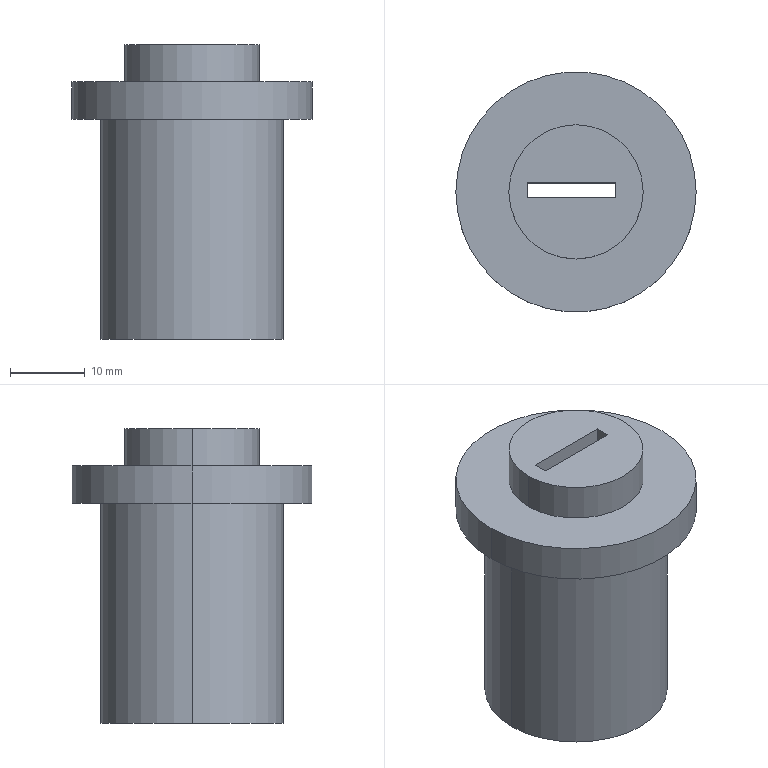Part | STEP file | 11-USB  11 | 1 solid | 14 faces | box 32.2 x 32.2 x 39.5 mm | volume 18221 mm3 | plane 8 | cylinder 6 | commonest cylinder face diameters 18 x2 24.4 x2 32.2 x2
STEP:
#1=CARTESIAN_POINT('',(9.,0.,39.5));
#2=VERTEX_POINT('',#1);
#3=CARTESIAN_POINT('',(-9.,0.,39.5));
#4=VERTEX_POINT('',#3);
#5=CARTESIAN_POINT('',(0.,0.,39.5));
#6=DIRECTION('',(0.,0.,1.));
#7=DIRECTION('',(1.,0.,0.));
#8=AXIS2_PLACEMENT_3D('',#5,#6,#7);
#9=CIRCLE('',#8,9.);
#10=EDGE_CURVE('',#2,#4,#9,.T.);
#11=ORIENTED_EDGE('',*,*,#10,.F.);
#12=CARTESIAN_POINT('',(9.,0.,34.5));
#13=VERTEX_POINT('',#12);
#14=CARTESIAN_POINT('',(9.,0.,39.5));
#15=DIRECTION('',(0.,0.,-1.));
#16=VECTOR('',#15,1000.);
#17=LINE('',#14,#16);
#18=EDGE_CURVE('',#2,#13,#17,.T.);
#19=ORIENTED_EDGE('',*,*,#18,.T.);
#20=CARTESIAN_POINT('',(-9.,0.,34.5));
#21=VERTEX_POINT('',#20);
#22=CARTESIAN_POINT('',(0.,0.,34.5));
#23=DIRECTION('',(0.,0.,1.));
#24=DIRECTION('',(1.,0.,0.));
#25=AXIS2_PLACEMENT_3D('',#22,#23,#24);
#26=CIRCLE('',#25,9.);
#27=EDGE_CURVE('',#13,#21,#26,.T.);
#28=ORIENTED_EDGE('',*,*,#27,.T.);
#29=CARTESIAN_POINT('',(-9.,0.,39.5));
#30=DIRECTION('',(0.,0.,-1.));
#31=VECTOR('',#30,1000.);
#32=LINE('',#29,#31);
#33=EDGE_CURVE('',#4,#21,#32,.T.);
#34=ORIENTED_EDGE('',*,*,#33,.F.);
#35=EDGE_LOOP('',(#11,#19,#28,#34));
#36=FACE_OUTER_BOUND('',#35,.T.);
#37=CARTESIAN_POINT('',(0.,0.,39.5));
#38=DIRECTION('',(0.,0.,-1.));
#39=DIRECTION('',(-1.,0.,0.));
#40=AXIS2_PLACEMENT_3D('',#37,#38,#39);
#41=CYLINDRICAL_SURFACE('',#40,9.);
#42=ADVANCED_FACE('',(#36),#41,.T.);
#43=CARTESIAN_POINT('',(16.1,0.,34.5));
#44=VERTEX_POINT('',#43);
#45=CARTESIAN_POINT('',(-16.1,0.,34.5));
#46=VERTEX_POINT('',#45);
#47=CARTESIAN_POINT('',(0.,0.,34.5));
#48=DIRECTION('',(0.,0.,1.));
#49=DIRECTION('',(1.,0.,0.));
#50=AXIS2_PLACEMENT_3D('',#47,#48,#49);
#51=CIRCLE('',#50,16.1);
#52=EDGE_CURVE('',#44,#46,#51,.T.);
#53=ORIENTED_EDGE('',*,*,#52,.F.);
#54=CARTESIAN_POINT('',(16.1,0.,29.5));
#55=VERTEX_POINT('',#54);
#56=CARTESIAN_POINT('',(16.1,0.,34.5));
#57=DIRECTION('',(0.,0.,-1.));
#58=VECTOR('',#57,1000.);
#59=LINE('',#56,#58);
#60=EDGE_CURVE('',#44,#55,#59,.T.);
#61=ORIENTED_EDGE('',*,*,#60,.T.);
#62=CARTESIAN_POINT('',(-16.1,0.,29.5));
#63=VERTEX_POINT('',#62);
#64=CARTESIAN_POINT('',(0.,0.,29.5));
#65=DIRECTION('',(0.,0.,1.));
#66=DIRECTION('',(1.,0.,0.));
#67=AXIS2_PLACEMENT_3D('',#64,#65,#66);
#68=CIRCLE('',#67,16.1);
#69=EDGE_CURVE('',#55,#63,#68,.T.);
#70=ORIENTED_EDGE('',*,*,#69,.T.);
#71=CARTESIAN_POINT('',(-16.1,0.,34.5));
#72=DIRECTION('',(0.,0.,-1.));
#73=VECTOR('',#72,1000.);
#74=LINE('',#71,#73);
#75=EDGE_CURVE('',#46,#63,#74,.T.);
#76=ORIENTED_EDGE('',*,*,#75,.F.);
#77=EDGE_LOOP('',(#53,#61,#70,#76));
#78=FACE_OUTER_BOUND('',#77,.T.);
#79=CARTESIAN_POINT('',(0.,0.,34.5));
#80=DIRECTION('',(0.,0.,-1.));
#81=DIRECTION('',(-1.,0.,0.));
#82=AXIS2_PLACEMENT_3D('',#79,#80,#81);
#83=CYLINDRICAL_SURFACE('',#82,16.1);
#84=ADVANCED_FACE('',(#78),#83,.T.);
#85=CARTESIAN_POINT('',(12.2,0.,29.5));
#86=VERTEX_POINT('',#85);
#87=CARTESIAN_POINT('',(-12.2,0.,29.5));
#88=VERTEX_POINT('',#87);
#89=CARTESIAN_POINT('',(0.,0.,29.5));
#90=DIRECTION('',(0.,0.,1.));
#91=DIRECTION('',(1.,0.,0.));
#92=AXIS2_PLACEMENT_3D('',#89,#90,#91);
#93=CIRCLE('',#92,12.2);
#94=EDGE_CURVE('',#86,#88,#93,.T.);
#95=ORIENTED_EDGE('',*,*,#94,.F.);
#96=CARTESIAN_POINT('',(12.2,0.,0.));
#97=VERTEX_POINT('',#96);
#98=CARTESIAN_POINT('',(12.2,0.,29.5));
#99=DIRECTION('',(0.,0.,-1.));
#100=VECTOR('',#99,1000.);
#101=LINE('',#98,#100);
#102=EDGE_CURVE('',#86,#97,#101,.T.);
#103=ORIENTED_EDGE('',*,*,#102,.T.);
#104=CARTESIAN_POINT('',(-12.2,0.,0.));
#105=VERTEX_POINT('',#104);
#106=CARTESIAN_POINT('',(0.,0.,0.));
#107=DIRECTION('',(0.,0.,1.));
#108=DIRECTION('',(1.,0.,0.));
#109=AXIS2_PLACEMENT_3D('',#106,#107,#108);
#110=CIRCLE('',#109,12.2);
#111=EDGE_CURVE('',#97,#105,#110,.T.);
#112=ORIENTED_EDGE('',*,*,#111,.T.);
#113=CARTESIAN_POINT('',(-12.2,0.,29.5));
#114=DIRECTION('',(0.,0.,-1.));
#115=VECTOR('',#114,1000.);
#116=LINE('',#113,#115);
#117=EDGE_CURVE('',#88,#105,#116,.T.);
#118=ORIENTED_EDGE('',*,*,#117,.F.);
#119=EDGE_LOOP('',(#95,#103,#112,#118));
#120=FACE_OUTER_BOUND('',#119,.T.);
#121=CARTESIAN_POINT('',(0.,0.,29.5));
#122=DIRECTION('',(0.,0.,-1.));
#123=DIRECTION('',(-1.,0.,0.));
#124=AXIS2_PLACEMENT_3D('',#121,#122,#123);
#125=CYLINDRICAL_SURFACE('',#124,12.2);
#126=ADVANCED_FACE('',(#120),#125,.T.);
#127=ORIENTED_EDGE('',*,*,#102,.F.);
#128=CARTESIAN_POINT('',(0.,0.,29.5));
#129=DIRECTION('',(0.,0.,1.));
#130=DIRECTION('',(1.,0.,0.));
#131=AXIS2_PLACEMENT_3D('',#128,#129,#130);
#132=CIRCLE('',#131,12.2);
#133=EDGE_CURVE('',#88,#86,#132,.T.);
#134=ORIENTED_EDGE('',*,*,#133,.F.);
#135=ORIENTED_EDGE('',*,*,#117,.T.);
#136=CARTESIAN_POINT('',(0.,0.,0.));
#137=DIRECTION('',(0.,0.,1.));
#138=DIRECTION('',(1.,0.,0.));
#139=AXIS2_PLACEMENT_3D('',#136,#137,#138);
#140=CIRCLE('',#139,12.2);
#141=EDGE_CURVE('',#105,#97,#140,.T.);
#142=ORIENTED_EDGE('',*,*,#141,.T.);
#143=EDGE_LOOP('',(#127,#134,#135,#142));
#144=FACE_OUTER_BOUND('',#143,.T.);
#145=CARTESIAN_POINT('',(0.,0.,29.5));
#146=DIRECTION('',(0.,0.,-1.));
#147=DIRECTION('',(-1.,0.,0.));
#148=AXIS2_PLACEMENT_3D('',#145,#146,#147);
#149=CYLINDRICAL_SURFACE('',#148,12.2);
#150=ADVANCED_FACE('',(#144),#149,.T.);
#151=CARTESIAN_POINT('',(5.32,-0.7338,0.));
#152=VERTEX_POINT('',#151);
#153=CARTESIAN_POINT('',(-6.543,-0.7338,0.));
#154=VERTEX_POINT('',#153);
#155=CARTESIAN_POINT('',(5.32,-0.7338,0.));
#156=DIRECTION('',(-1.,0.,0.));
#157=VECTOR('',#156,1000.);
#158=LINE('',#155,#157);
#159=EDGE_CURVE('',#152,#154,#158,.T.);
#160=ORIENTED_EDGE('',*,*,#159,.F.);
#161=CARTESIAN_POINT('',(5.32,1.223,0.));
#162=VERTEX_POINT('',#161);
#163=CARTESIAN_POINT('',(5.32,1.223,0.));
#164=DIRECTION('',(0.,-1.,0.));
#165=VECTOR('',#164,1000.);
#166=LINE('',#163,#165);
#167=EDGE_CURVE('',#162,#152,#166,.T.);
#168=ORIENTED_EDGE('',*,*,#167,.F.);
#169=CARTESIAN_POINT('',(-6.543,1.223,0.));
#170=VERTEX_POINT('',#169);
#171=CARTESIAN_POINT('',(5.32,1.223,0.));
#172=DIRECTION('',(1.,0.,0.));
#173=VECTOR('',#172,1000.);
#174=LINE('',#171,#173);
#175=EDGE_CURVE('',#170,#162,#174,.T.);
#176=ORIENTED_EDGE('',*,*,#175,.F.);
#177=CARTESIAN_POINT('',(-6.543,1.223,0.));
#178=DIRECTION('',(0.,1.,0.));
#179=VECTOR('',#178,1000.);
#180=LINE('',#177,#179);
#181=EDGE_CURVE('',#154,#170,#180,.T.);
#182=ORIENTED_EDGE('',*,*,#181,.F.);
#183=EDGE_LOOP('',(#160,#168,#176,#182));
#184=FACE_BOUND('',#183,.T.);
#185=ORIENTED_EDGE('',*,*,#141,.F.);
#186=ORIENTED_EDGE('',*,*,#111,.F.);
#187=EDGE_LOOP('',(#185,#186));
#188=FACE_OUTER_BOUND('',#187,.T.);
#189=CARTESIAN_POINT('',(0.,0.,0.));
#190=DIRECTION('',(0.,0.,1.));
#191=DIRECTION('',(1.,0.,0.));
#192=AXIS2_PLACEMENT_3D('',#189,#190,#191);
#193=PLANE('',#192);
#194=ADVANCED_FACE('',(#184,#188),#193,.F.);
#195=ORIENTED_EDGE('',*,*,#60,.F.);
#196=CARTESIAN_POINT('',(0.,0.,34.5));
#197=DIRECTION('',(0.,0.,1.));
#198=DIRECTION('',(1.,0.,0.));
#199=AXIS2_PLACEMENT_3D('',#196,#197,#198);
#200=CIRCLE('',#199,16.1);
#201=EDGE_CURVE('',#46,#44,#200,.T.);
#202=ORIENTED_EDGE('',*,*,#201,.F.);
#203=ORIENTED_EDGE('',*,*,#75,.T.);
#204=CARTESIAN_POINT('',(0.,0.,29.5));
#205=DIRECTION('',(0.,0.,1.));
#206=DIRECTION('',(1.,0.,0.));
#207=AXIS2_PLACEMENT_3D('',#204,#205,#206);
#208=CIRCLE('',#207,16.1);
#209=EDGE_CURVE('',#63,#55,#208,.T.);
#210=ORIENTED_EDGE('',*,*,#209,.T.);
#211=EDGE_LOOP('',(#195,#202,#203,#210));
#212=FACE_OUTER_BOUND('',#211,.T.);
#213=CARTESIAN_POINT('',(0.,0.,34.5));
#214=DIRECTION('',(0.,0.,-1.));
#215=DIRECTION('',(-1.,0.,0.));
#216=AXIS2_PLACEMENT_3D('',#213,#214,#215);
#217=CYLINDRICAL_SURFACE('',#216,16.1);
#218=ADVANCED_FACE('',(#212),#217,.T.);
#219=CARTESIAN_POINT('',(0.,0.,34.5));
#220=DIRECTION('',(0.,0.,1.));
#221=DIRECTION('',(1.,0.,0.));
#222=AXIS2_PLACEMENT_3D('',#219,#220,#221);
#223=CIRCLE('',#222,9.);
#224=EDGE_CURVE('',#21,#13,#223,.T.);
#225=ORIENTED_EDGE('',*,*,#224,.F.);
#226=ORIENTED_EDGE('',*,*,#27,.F.);
#227=EDGE_LOOP('',(#225,#226));
#228=FACE_BOUND('',#227,.T.);
#229=ORIENTED_EDGE('',*,*,#201,.T.);
#230=ORIENTED_EDGE('',*,*,#52,.T.);
#231=EDGE_LOOP('',(#229,#230));
#232=FACE_OUTER_BOUND('',#231,.T.);
#233=CARTESIAN_POINT('',(0.,0.,34.5));
#234=DIRECTION('',(0.,0.,1.));
#235=DIRECTION('',(1.,0.,0.));
#236=AXIS2_PLACEMENT_3D('',#233,#234,#235);
#237=PLANE('',#236);
#238=ADVANCED_FACE('',(#228,#232),#237,.T.);
#239=ORIENTED_EDGE('',*,*,#133,.T.);
#240=ORIENTED_EDGE('',*,*,#94,.T.);
#241=EDGE_LOOP('',(#239,#240));
#242=FACE_BOUND('',#241,.T.);
#243=ORIENTED_EDGE('',*,*,#209,.F.);
#244=ORIENTED_EDGE('',*,*,#69,.F.);
#245=EDGE_LOOP('',(#243,#244));
#246=FACE_OUTER_BOUND('',#245,.T.);
#247=CARTESIAN_POINT('',(0.,0.,29.5));
#248=DIRECTION('',(0.,0.,1.));
#249=DIRECTION('',(1.,0.,0.));
#250=AXIS2_PLACEMENT_3D('',#247,#248,#249);
#251=PLANE('',#250);
#252=ADVANCED_FACE('',(#242,#246),#251,.F.);
#253=ORIENTED_EDGE('',*,*,#18,.F.);
#254=CARTESIAN_POINT('',(0.,0.,39.5));
#255=DIRECTION('',(0.,0.,1.));
#256=DIRECTION('',(1.,0.,0.));
#257=AXIS2_PLACEMENT_3D('',#254,#255,#256);
#258=CIRCLE('',#257,9.);
#259=EDGE_CURVE('',#4,#2,#258,.T.);
#260=ORIENTED_EDGE('',*,*,#259,.F.);
#261=ORIENTED_EDGE('',*,*,#33,.T.);
#262=ORIENTED_EDGE('',*,*,#224,.T.);
#263=EDGE_LOOP('',(#253,#260,#261,#262));
#264=FACE_OUTER_BOUND('',#263,.T.);
#265=CARTESIAN_POINT('',(0.,0.,39.5));
#266=DIRECTION('',(0.,0.,-1.));
#267=DIRECTION('',(-1.,0.,0.));
#268=AXIS2_PLACEMENT_3D('',#265,#266,#267);
#269=CYLINDRICAL_SURFACE('',#268,9.);
#270=ADVANCED_FACE('',(#264),#269,.T.);
#271=CARTESIAN_POINT('',(5.32,1.223,39.5));
#272=VERTEX_POINT('',#271);
#273=CARTESIAN_POINT('',(5.32,-0.7338,39.5));
#274=VERTEX_POINT('',#273);
#275=CARTESIAN_POINT('',(5.32,1.223,39.5));
#276=DIRECTION('',(0.,-1.,0.));
#277=VECTOR('',#276,1000.);
#278=LINE('',#275,#277);
#279=EDGE_CURVE('',#272,#274,#278,.T.);
#280=ORIENTED_EDGE('',*,*,#279,.T.);
#281=CARTESIAN_POINT('',(-6.543,-0.7338,39.5));
#282=VERTEX_POINT('',#281);
#283=CARTESIAN_POINT('',(5.32,-0.7338,39.5));
#284=DIRECTION('',(-1.,0.,0.));
#285=VECTOR('',#284,1000.);
#286=LINE('',#283,#285);
#287=EDGE_CURVE('',#274,#282,#286,.T.);
#288=ORIENTED_EDGE('',*,*,#287,.T.);
#289=CARTESIAN_POINT('',(-6.543,1.223,39.5));
#290=VERTEX_POINT('',#289);
#291=CARTESIAN_POINT('',(-6.543,1.223,39.5));
#292=DIRECTION('',(0.,1.,0.));
#293=VECTOR('',#292,1000.);
#294=LINE('',#291,#293);
#295=EDGE_CURVE('',#282,#290,#294,.T.);
#296=ORIENTED_EDGE('',*,*,#295,.T.);
#297=CARTESIAN_POINT('',(5.32,1.223,39.5));
#298=DIRECTION('',(1.,0.,0.));
#299=VECTOR('',#298,1000.);
#300=LINE('',#297,#299);
#301=EDGE_CURVE('',#290,#272,#300,.T.);
#302=ORIENTED_EDGE('',*,*,#301,.T.);
#303=EDGE_LOOP('',(#280,#288,#296,#302));
#304=FACE_BOUND('',#303,.T.);
#305=ORIENTED_EDGE('',*,*,#259,.T.);
#306=ORIENTED_EDGE('',*,*,#10,.T.);
#307=EDGE_LOOP('',(#305,#306));
#308=FACE_OUTER_BOUND('',#307,.T.);
#309=CARTESIAN_POINT('',(0.,0.,39.5));
#310=DIRECTION('',(0.,0.,1.));
#311=DIRECTION('',(1.,0.,0.));
#312=AXIS2_PLACEMENT_3D('',#309,#310,#311);
#313=PLANE('',#312);
#314=ADVANCED_FACE('',(#304,#308),#313,.T.);
#315=ORIENTED_EDGE('',*,*,#167,.T.);
#316=CARTESIAN_POINT('',(5.32,-0.7338,39.5));
#317=DIRECTION('',(0.,0.,-1.));
#318=VECTOR('',#317,1000.);
#319=LINE('',#316,#318);
#320=EDGE_CURVE('',#274,#152,#319,.T.);
#321=ORIENTED_EDGE('',*,*,#320,.F.);
#322=ORIENTED_EDGE('',*,*,#279,.F.);
#323=CARTESIAN_POINT('',(5.32,1.223,39.5));
#324=DIRECTION('',(0.,0.,-1.));
#325=VECTOR('',#324,1000.);
#326=LINE('',#323,#325);
#327=EDGE_CURVE('',#272,#162,#326,.T.);
#328=ORIENTED_EDGE('',*,*,#327,.T.);
#329=EDGE_LOOP('',(#315,#321,#322,#328));
#330=FACE_OUTER_BOUND('',#329,.T.);
#331=CARTESIAN_POINT('',(5.32,1.223,39.5));
#332=DIRECTION('',(1.,0.,0.));
#333=DIRECTION('',(0.,0.,-1.));
#334=AXIS2_PLACEMENT_3D('',#331,#332,#333);
#335=PLANE('',#334);
#336=ADVANCED_FACE('',(#330),#335,.F.);
#337=ORIENTED_EDGE('',*,*,#175,.T.);
#338=ORIENTED_EDGE('',*,*,#327,.F.);
#339=ORIENTED_EDGE('',*,*,#301,.F.);
#340=CARTESIAN_POINT('',(-6.543,1.223,39.5));
#341=DIRECTION('',(0.,0.,-1.));
#342=VECTOR('',#341,1000.);
#343=LINE('',#340,#342);
#344=EDGE_CURVE('',#290,#170,#343,.T.);
#345=ORIENTED_EDGE('',*,*,#344,.T.);
#346=EDGE_LOOP('',(#337,#338,#339,#345));
#347=FACE_OUTER_BOUND('',#346,.T.);
#348=CARTESIAN_POINT('',(5.32,1.223,39.5));
#349=DIRECTION('',(0.,1.,0.));
#350=DIRECTION('',(0.,0.,1.));
#351=AXIS2_PLACEMENT_3D('',#348,#349,#350);
#352=PLANE('',#351);
#353=ADVANCED_FACE('',(#347),#352,.F.);
#354=ORIENTED_EDGE('',*,*,#181,.T.);
#355=ORIENTED_EDGE('',*,*,#344,.F.);
#356=ORIENTED_EDGE('',*,*,#295,.F.);
#357=CARTESIAN_POINT('',(-6.543,-0.7338,39.5));
#358=DIRECTION('',(0.,0.,-1.));
#359=VECTOR('',#358,1000.);
#360=LINE('',#357,#359);
#361=EDGE_CURVE('',#282,#154,#360,.T.);
#362=ORIENTED_EDGE('',*,*,#361,.T.);
#363=EDGE_LOOP('',(#354,#355,#356,#362));
#364=FACE_OUTER_BOUND('',#363,.T.);
#365=CARTESIAN_POINT('',(-6.543,1.223,39.5));
#366=DIRECTION('',(-1.,0.,0.));
#367=DIRECTION('',(0.,-1.,0.));
#368=AXIS2_PLACEMENT_3D('',#365,#366,#367);
#369=PLANE('',#368);
#370=ADVANCED_FACE('',(#364),#369,.F.);
#371=ORIENTED_EDGE('',*,*,#159,.T.);
#372=ORIENTED_EDGE('',*,*,#361,.F.);
#373=ORIENTED_EDGE('',*,*,#287,.F.);
#374=ORIENTED_EDGE('',*,*,#320,.T.);
#375=EDGE_LOOP('',(#371,#372,#373,#374));
#376=FACE_OUTER_BOUND('',#375,.T.);
#377=CARTESIAN_POINT('',(5.32,-0.7338,39.5));
#378=DIRECTION('',(0.,-1.,0.));
#379=DIRECTION('',(0.,0.,-1.));
#380=AXIS2_PLACEMENT_3D('',#377,#378,#379);
#381=PLANE('',#380);
#382=ADVANCED_FACE('',(#376),#381,.F.);
#383=CLOSED_SHELL('',(#42,#84,#126,#150,#194,#218,#238,#252,#270,#314,#336,#353,#370,#382));
#384=MANIFOLD_SOLID_BREP('',#383);
#385=CARTESIAN_POINT('',(0.,0.,0.));
#386=DIRECTION('',(0.,0.,1.));
#387=DIRECTION('',(1.,0.,0.));
#388=AXIS2_PLACEMENT_3D('',#385,#386,#387);
#389=(LENGTH_UNIT()NAMED_UNIT(*)SI_UNIT(.MILLI.,.METRE.));
#390=UNCERTAINTY_MEASURE_WITH_UNIT(LENGTH_MEASURE(0.00001),#389,'','');
#391=(NAMED_UNIT(*)PLANE_ANGLE_UNIT()SI_UNIT($,.RADIAN.));
#392=(NAMED_UNIT(*)SI_UNIT($,.STERADIAN.)SOLID_ANGLE_UNIT());
#393=(GEOMETRIC_REPRESENTATION_CONTEXT(3)GLOBAL_UNCERTAINTY_ASSIGNED_CONTEXT((#390))GLOBAL_UNIT_ASSIGNED_CONTEXT((#389,#391,#392))REPRESENTATION_CONTEXT('',''));
#394=ADVANCED_BREP_SHAPE_REPRESENTATION('',(#384,#388),#393);